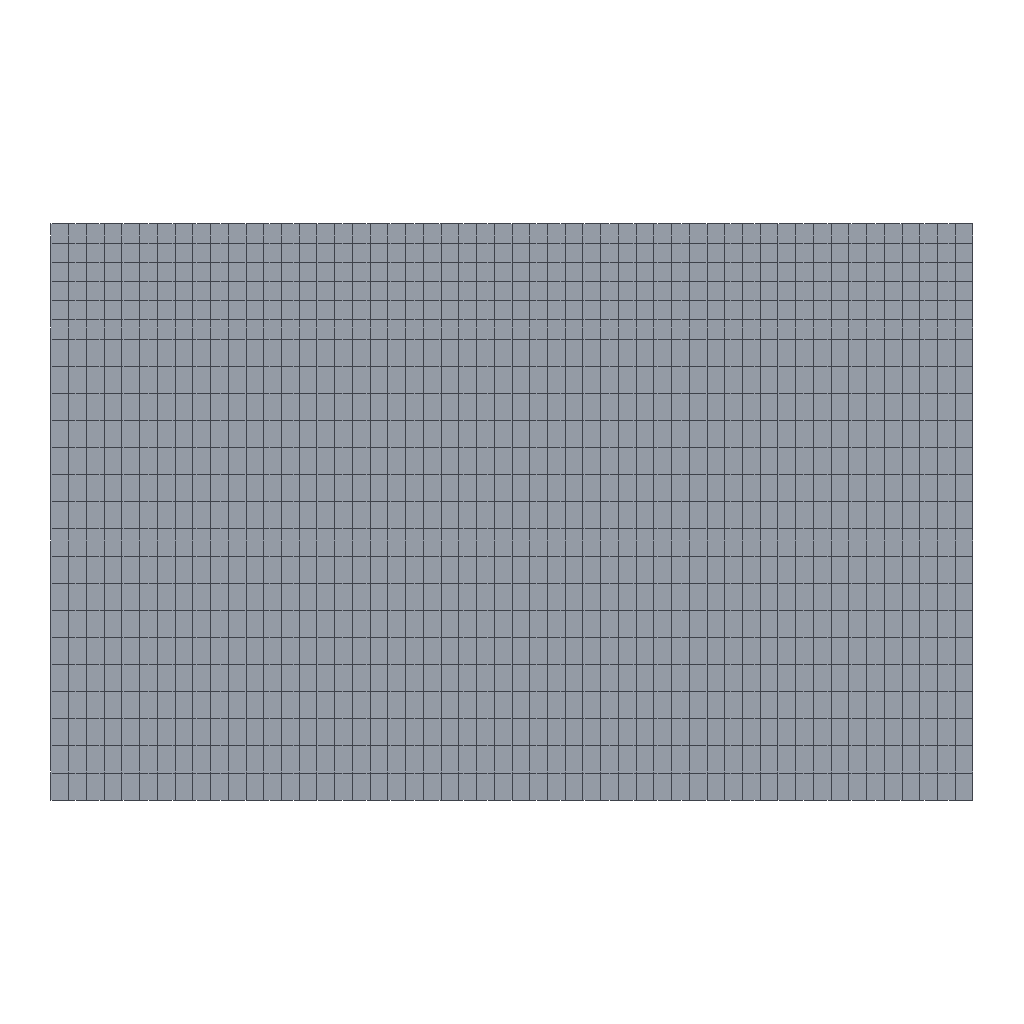Simulation study | abaqus
Set-up summary:
category,name,step,type,value,unit,region
solver,abaqus
solver,version,,,Abaqus/Standard 2020
units,not stated in the deck,,not stated
analysis,deck,,static,static
load_step,Step-1,Step-1,static
load_step,requested,,,1
mesh,nodes,,,1272
mesh,elements,,,1196
element_type,CPS4R,,plane,1196
load,load commands in deck,,count,52
bc,support commands in deck,,count,1
material,JITI,,in results
material,TUCENG,,in results
check,setup vs results,,match,"per instance, exact: element labels, types and connectivity; labels of the nodes the elements use; coordinates of those nodes at SINGLE_PRECISION in 1 of 1 instance(s)"
Abaqus input file, long lists of numbers shortened:
*Heading
** Job name: Job-1 Model name: Model-1
** Generated by: Abaqus/CAE 2020
*Preprint, echo=NO, model=NO, history=NO, contact=NO
**
** PARTS
**
*Part, name=Part-1
*Node
      1,           1.,       -0.125
      2,           0.,       -0.125
** (1270 more lines like these left out)
*Element, type=CPS4R
  1,    1,   10,  202,  143
  2,   10,   11,  203,  202
** (1194 more lines like these left out)
*Nset, nset=Set-3
    1,    2,    5,    6,    7,    8,    9,   10,   11,   12,   13,   14,   15,   16,   17,   18
   19,   20,   21,   22,   23,   24,   25,   26,   27,   28,   29,   30,   31,   32,   33,   34
** (22 more lines like these left out)
*Elset, elset=Set-3, generate
  885,  1196,     1
*Nset, nset=Set-4
    1,    2,    3,    4,   10,   11,   12,   13,   14,   15,   16,   17,   18,   19,   20,   21
   22,   23,   24,   25,   26,   27,   28,   29,   30,   31,   32,   33,   34,   35,   36,   37
** (58 more lines like these left out)
*Elset, elset=Set-4, generate
   1,  884,    1
** Section: jiti
*Solid Section, elset=Set-4, material=jiti
,
** Section: teceng
*Solid Section, elset=Set-3, material=tuceng
,
*End Part
**
**
** ASSEMBLY
**
*Assembly, name=Assembly
**
*Instance, name=Part-1-1, part=Part-1
        -0.5,           0.,           0.
*End Instance
**
*Nset, nset=Set-1, instance=Part-1-1
   1,   2,   3,   4,  61,  62,  63,  64,  65,  66,  67,  68,  69,  70,  71,  72
  73,  74,  75,  76,  77,  78,  79,  80,  81,  82,  83,  84,  85,  86,  87,  88
** (4 more lines like these left out)
*Elset, elset=Set-1, instance=Part-1-1
   1,  52,  53, 104, 105, 156, 157, 208, 209, 260, 261, 312, 313, 364, 365, 416
 417, 468, 469, 520, 521, 572, 573, 624, 625, 676, 677, 728, 729, 780, 781, 832
** (4 more lines like these left out)
*Nset, nset=Set-2, instance=Part-1-1
   1,   2,   3,   4,   8,   9,  61,  62,  63,  64,  65,  66,  67,  68,  69,  70
  71,  72,  73,  74,  75,  76,  77,  78,  79,  80,  81,  82,  83,  84,  85,  86
** (5 more lines like these left out)
*Elset, elset=Set-2, instance=Part-1-1
    1,   52,   53,  104,  105,  156,  157,  208,  209,  260,  261,  312,  313,  364,  365,  416
  417,  468,  469,  520,  521,  572,  573,  624,  625,  676,  677,  728,  729,  780,  781,  832
** (4 more lines like these left out)
*Elset, elset=_Surf-3_S3, internal, instance=Part-1-1, generate
 1158,  1183,     1
*Surface, type=ELEMENT, name=Surf-3
_Surf-3_S3, S3
*Elset, elset=_Surf-4_S3, internal, instance=Part-1-1, generate
 1158,  1183,     1
*Surface, type=ELEMENT, name=Surf-4
_Surf-4_S3, S3
*End Assembly
*Amplitude, name=Amp-1
             0.,              0.,              1.,              1.
**
** MATERIALS
**
*Material, name=jiti
*Elastic
21000., 0.3
*Material, name=tuceng
*Elastic
475000., 0.22
** ----------------------------------------------------------------
**
** STEP: Step-1
**
*Step, name=Step-1, nlgeom=YES, inc=1000
*Static, stabilize=0.0002, allsdtol=0.05, continue=NO
0.01, 1., 1e-05, 1.
**
** BOUNDARY CONDITIONS
**
** Name: BC-1 Type: 对称/反对称/完全固定
*Boundary
Set-2, ENCASTRE
**
** LOADS
**
** Name: Load-1   Type: Surface traction Using Field: AnalyticalField-1
*Dload, amplitude=Amp-1
Part-1-1.117, TRVEC3, 92.046, 1., 0., 0.
Part-1-1.117, TRVEC3, 92.012, 1., 0., 0.
Part-1-1.117, TRVEC3, 91.944, 1., 0., 0.
Part-1-1.117, TRVEC3, 91.841, 1., 0., 0.
Part-1-1.117, TRVEC3, 91.705, 1., 0., 0.
Part-1-1.118, TRVEC3, 91.534, 1., 0., 0.
Part-1-1.118, TRVEC3, 91.328, 1., 0., 0.
Part-1-1.118, TRVEC3, 91.088, 1., 0., 0.
Part-1-1.118, TRVEC3, 90.812, 1., 0., 0.
Part-1-1.118, TRVEC3, 90.501, 1., 0., 0.
Part-1-1.118, TRVEC3, 90.154, 1., 0., 0.
Part-1-1.118, TRVEC3, 89.771, 1., 0., 0.
Part-1-1.118, TRVEC3, 89.351, 1., 0., 0.
Part-1-1.116, TRVEC3, 89.351, 1., 0., 0.
Part-1-1.116, TRVEC3, 89.771, 1., 0., 0.
Part-1-1.116, TRVEC3, 90.154, 1., 0., 0.
Part-1-1.116, TRVEC3, 90.501, 1., 0., 0.
Part-1-1.116, TRVEC3, 90.812, 1., 0., 0.
Part-1-1.116, TRVEC3, 91.088, 1., 0., 0.
Part-1-1.116, TRVEC3, 91.328, 1., 0., 0.
Part-1-1.117, TRVEC3, 91.534, 1., 0., 0.
Part-1-1.117, TRVEC3, 91.705, 1., 0., 0.
Part-1-1.117, TRVEC3, 91.841, 1., 0., 0.
Part-1-1.117, TRVEC3, 91.944, 1., 0., 0.
Part-1-1.117, TRVEC3, 92.012, 1., 0., 0.
Part-1-1.117, TRVEC3, 92.046, 1., 0., 0.
** Name: Load-2   Type: Pressure Using Field: AnalyticalField-1
*Dload, amplitude=Amp-1
Part-1-1.117, P3, 1840.91
Part-1-1.117, P3, 1840.23
Part-1-1.117, P3, 1838.87
Part-1-1.117, P3, 1836.83
Part-1-1.117, P3, 1834.09
Part-1-1.118, P3, 1830.67
Part-1-1.118, P3, 1826.56
Part-1-1.118, P3, 1821.75
Part-1-1.118, P3, 1816.24
Part-1-1.118, P3, 1810.02
Part-1-1.118, P3, 1803.08
Part-1-1.118, P3, 1795.41
Part-1-1.118, P3, 1787.02
Part-1-1.116, P3, 1787.02
Part-1-1.116, P3, 1795.41
Part-1-1.116, P3, 1803.08
Part-1-1.116, P3, 1810.02
Part-1-1.116, P3, 1816.24
Part-1-1.116, P3, 1821.75
Part-1-1.116, P3, 1826.56
Part-1-1.117, P3, 1830.67
Part-1-1.117, P3, 1834.09
Part-1-1.117, P3, 1836.83
Part-1-1.117, P3, 1838.87
Part-1-1.117, P3, 1840.23
Part-1-1.117, P3, 1840.91
**
** OUTPUT REQUESTS
**
*Restart, write, frequency=0
**
** FIELD OUTPUT: F-Output-1
**
*Output, field
*Node Output
CF, RF, U, V
*Element Output, directions=YES
E, LE, MISES, MISESMAX, PE, PEEQ, PEMAG, S
*Contact Output
CDISP, CSTRESS
**
** HISTORY OUTPUT: H-Output-1
**
*Output, history, variable=PRESELECT
*End Step
Results summary:
result,step,,completed,increments=11 time=1.0/1.0
result,analysis,,,static
result,last_loadstep,,,1
result,primary field,,,U
result,reaction total,,FX,-44.706,model units
result,reaction total,,FY,898.636,model units
result,reaction total,,FZ,0.0,model units